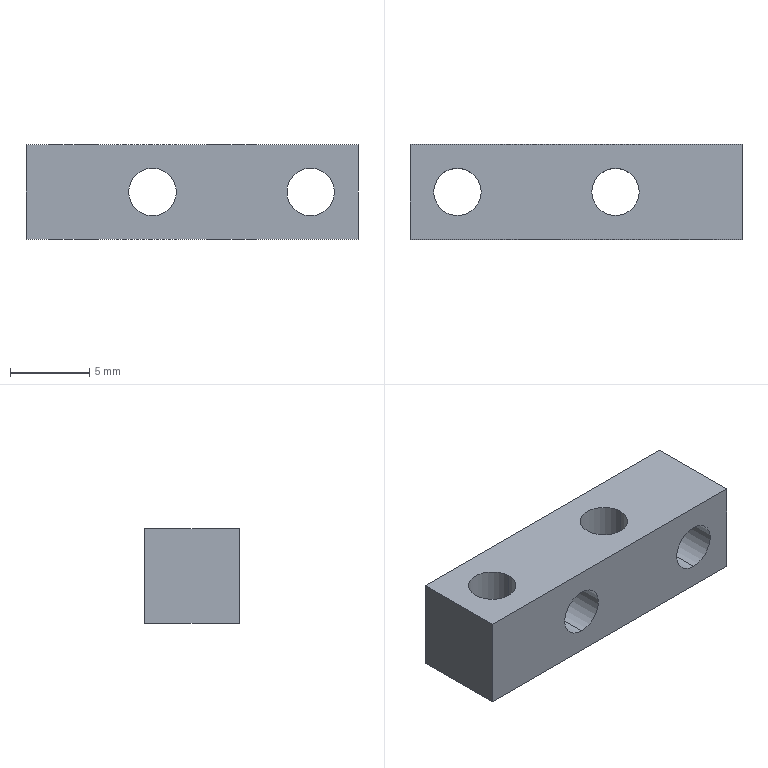Part | SolidWorks | features Extrusion 1, ICE 1 | 1 solid | 14 faces | box 21 x 6 x 6 mm | volume 586.354 mm3 | cylinder 8 | plane 6 | commonest cylinder face diameters 3 x8
STEP:
#1=CARTESIAN_POINT('',(8.,0.,1.5));
#2=VERTEX_POINT('',#1);
#3=CARTESIAN_POINT('',(8.,0.,4.5));
#4=VERTEX_POINT('',#3);
#5=CARTESIAN_POINT('',(8.,0.,3.));
#6=DIRECTION('',(0.,1.,0.));
#7=DIRECTION('',(0.,0.,1.));
#8=AXIS2_PLACEMENT_3D('',#5,#6,#7);
#9=CIRCLE('',#8,1.5);
#10=EDGE_CURVE('',#2,#4,#9,.T.);
#11=ORIENTED_EDGE('',*,*,#10,.F.);
#12=CARTESIAN_POINT('',(8.,6.,1.5));
#13=VERTEX_POINT('',#12);
#14=CARTESIAN_POINT('',(8.,0.,1.5));
#15=DIRECTION('',(0.,1.,0.));
#16=VECTOR('',#15,1000.);
#17=LINE('',#14,#16);
#18=EDGE_CURVE('',#2,#13,#17,.T.);
#19=ORIENTED_EDGE('',*,*,#18,.T.);
#20=CARTESIAN_POINT('',(8.,6.,4.5));
#21=VERTEX_POINT('',#20);
#22=CARTESIAN_POINT('',(8.,6.,3.));
#23=DIRECTION('',(0.,-1.,0.));
#24=DIRECTION('',(0.,0.,-1.));
#25=AXIS2_PLACEMENT_3D('',#22,#23,#24);
#26=CIRCLE('',#25,1.5);
#27=EDGE_CURVE('',#21,#13,#26,.T.);
#28=ORIENTED_EDGE('',*,*,#27,.F.);
#29=CARTESIAN_POINT('',(8.,0.,4.5));
#30=DIRECTION('',(0.,1.,0.));
#31=VECTOR('',#30,1000.);
#32=LINE('',#29,#31);
#33=EDGE_CURVE('',#4,#21,#32,.T.);
#34=ORIENTED_EDGE('',*,*,#33,.F.);
#35=EDGE_LOOP('',(#11,#19,#28,#34));
#36=FACE_OUTER_BOUND('',#35,.T.);
#37=CARTESIAN_POINT('',(8.,0.,3.));
#38=DIRECTION('',(0.,1.,0.));
#39=DIRECTION('',(0.,0.,1.));
#40=AXIS2_PLACEMENT_3D('',#37,#38,#39);
#41=CYLINDRICAL_SURFACE('',#40,1.5);
#42=ADVANCED_FACE('',(#36),#41,.F.);
#43=CARTESIAN_POINT('',(18.,0.,1.5));
#44=VERTEX_POINT('',#43);
#45=CARTESIAN_POINT('',(18.,0.,4.5));
#46=VERTEX_POINT('',#45);
#47=CARTESIAN_POINT('',(18.,0.,3.));
#48=DIRECTION('',(0.,1.,0.));
#49=DIRECTION('',(0.,0.,1.));
#50=AXIS2_PLACEMENT_3D('',#47,#48,#49);
#51=CIRCLE('',#50,1.5);
#52=EDGE_CURVE('',#44,#46,#51,.T.);
#53=ORIENTED_EDGE('',*,*,#52,.F.);
#54=CARTESIAN_POINT('',(18.,6.,1.5));
#55=VERTEX_POINT('',#54);
#56=CARTESIAN_POINT('',(18.,0.,1.5));
#57=DIRECTION('',(0.,1.,0.));
#58=VECTOR('',#57,1000.);
#59=LINE('',#56,#58);
#60=EDGE_CURVE('',#44,#55,#59,.T.);
#61=ORIENTED_EDGE('',*,*,#60,.T.);
#62=CARTESIAN_POINT('',(18.,6.,4.5));
#63=VERTEX_POINT('',#62);
#64=CARTESIAN_POINT('',(18.,6.,3.));
#65=DIRECTION('',(0.,-1.,0.));
#66=DIRECTION('',(0.,0.,-1.));
#67=AXIS2_PLACEMENT_3D('',#64,#65,#66);
#68=CIRCLE('',#67,1.5);
#69=EDGE_CURVE('',#63,#55,#68,.T.);
#70=ORIENTED_EDGE('',*,*,#69,.F.);
#71=CARTESIAN_POINT('',(18.,0.,4.5));
#72=DIRECTION('',(0.,1.,0.));
#73=VECTOR('',#72,1000.);
#74=LINE('',#71,#73);
#75=EDGE_CURVE('',#46,#63,#74,.T.);
#76=ORIENTED_EDGE('',*,*,#75,.F.);
#77=EDGE_LOOP('',(#53,#61,#70,#76));
#78=FACE_OUTER_BOUND('',#77,.T.);
#79=CARTESIAN_POINT('',(18.,0.,3.));
#80=DIRECTION('',(0.,1.,0.));
#81=DIRECTION('',(0.,0.,1.));
#82=AXIS2_PLACEMENT_3D('',#79,#80,#81);
#83=CYLINDRICAL_SURFACE('',#82,1.5);
#84=ADVANCED_FACE('',(#78),#83,.F.);
#85=CARTESIAN_POINT('',(11.5,3.,6.));
#86=VERTEX_POINT('',#85);
#87=CARTESIAN_POINT('',(14.5,3.,6.));
#88=VERTEX_POINT('',#87);
#89=CARTESIAN_POINT('',(13.,3.,6.));
#90=DIRECTION('',(0.,0.,1.));
#91=DIRECTION('',(1.,0.,0.));
#92=AXIS2_PLACEMENT_3D('',#89,#90,#91);
#93=CIRCLE('',#92,1.5);
#94=EDGE_CURVE('',#86,#88,#93,.T.);
#95=ORIENTED_EDGE('',*,*,#94,.T.);
#96=CARTESIAN_POINT('',(14.5,3.,0.));
#97=VERTEX_POINT('',#96);
#98=CARTESIAN_POINT('',(14.5,3.,6.));
#99=DIRECTION('',(0.,0.,-1.));
#100=VECTOR('',#99,1000.);
#101=LINE('',#98,#100);
#102=EDGE_CURVE('',#88,#97,#101,.T.);
#103=ORIENTED_EDGE('',*,*,#102,.T.);
#104=CARTESIAN_POINT('',(11.5,3.,0.));
#105=VERTEX_POINT('',#104);
#106=CARTESIAN_POINT('',(13.,3.,0.));
#107=DIRECTION('',(0.,0.,1.));
#108=DIRECTION('',(1.,0.,0.));
#109=AXIS2_PLACEMENT_3D('',#106,#107,#108);
#110=CIRCLE('',#109,1.5);
#111=EDGE_CURVE('',#105,#97,#110,.T.);
#112=ORIENTED_EDGE('',*,*,#111,.F.);
#113=CARTESIAN_POINT('',(11.5,3.,6.));
#114=DIRECTION('',(0.,0.,-1.));
#115=VECTOR('',#114,1000.);
#116=LINE('',#113,#115);
#117=EDGE_CURVE('',#86,#105,#116,.T.);
#118=ORIENTED_EDGE('',*,*,#117,.F.);
#119=EDGE_LOOP('',(#95,#103,#112,#118));
#120=FACE_OUTER_BOUND('',#119,.T.);
#121=CARTESIAN_POINT('',(13.,3.,6.));
#122=DIRECTION('',(0.,0.,-1.));
#123=DIRECTION('',(-1.,0.,0.));
#124=AXIS2_PLACEMENT_3D('',#121,#122,#123);
#125=CYLINDRICAL_SURFACE('',#124,1.5);
#126=ADVANCED_FACE('',(#120),#125,.F.);
#127=CARTESIAN_POINT('',(1.5,3.,6.));
#128=VERTEX_POINT('',#127);
#129=CARTESIAN_POINT('',(4.5,3.,6.));
#130=VERTEX_POINT('',#129);
#131=CARTESIAN_POINT('',(3.,3.,6.));
#132=DIRECTION('',(0.,0.,1.));
#133=DIRECTION('',(1.,0.,0.));
#134=AXIS2_PLACEMENT_3D('',#131,#132,#133);
#135=CIRCLE('',#134,1.5);
#136=EDGE_CURVE('',#128,#130,#135,.T.);
#137=ORIENTED_EDGE('',*,*,#136,.T.);
#138=CARTESIAN_POINT('',(4.5,3.,0.));
#139=VERTEX_POINT('',#138);
#140=CARTESIAN_POINT('',(4.5,3.,6.));
#141=DIRECTION('',(0.,0.,-1.));
#142=VECTOR('',#141,1000.);
#143=LINE('',#140,#142);
#144=EDGE_CURVE('',#130,#139,#143,.T.);
#145=ORIENTED_EDGE('',*,*,#144,.T.);
#146=CARTESIAN_POINT('',(1.5,3.,0.));
#147=VERTEX_POINT('',#146);
#148=CARTESIAN_POINT('',(3.,3.,0.));
#149=DIRECTION('',(0.,0.,1.));
#150=DIRECTION('',(1.,0.,0.));
#151=AXIS2_PLACEMENT_3D('',#148,#149,#150);
#152=CIRCLE('',#151,1.5);
#153=EDGE_CURVE('',#147,#139,#152,.T.);
#154=ORIENTED_EDGE('',*,*,#153,.F.);
#155=CARTESIAN_POINT('',(1.5,3.,6.));
#156=DIRECTION('',(0.,0.,-1.));
#157=VECTOR('',#156,1000.);
#158=LINE('',#155,#157);
#159=EDGE_CURVE('',#128,#147,#158,.T.);
#160=ORIENTED_EDGE('',*,*,#159,.F.);
#161=EDGE_LOOP('',(#137,#145,#154,#160));
#162=FACE_OUTER_BOUND('',#161,.T.);
#163=CARTESIAN_POINT('',(3.,3.,6.));
#164=DIRECTION('',(0.,0.,-1.));
#165=DIRECTION('',(-1.,0.,0.));
#166=AXIS2_PLACEMENT_3D('',#163,#164,#165);
#167=CYLINDRICAL_SURFACE('',#166,1.5);
#168=ADVANCED_FACE('',(#162),#167,.F.);
#169=CARTESIAN_POINT('',(0.,6.,6.));
#170=VERTEX_POINT('',#169);
#171=CARTESIAN_POINT('',(0.,0.,6.));
#172=VERTEX_POINT('',#171);
#173=CARTESIAN_POINT('',(0.,0.,6.));
#174=DIRECTION('',(0.,-1.,0.));
#175=VECTOR('',#174,1000.);
#176=LINE('',#173,#175);
#177=EDGE_CURVE('',#170,#172,#176,.T.);
#178=ORIENTED_EDGE('',*,*,#177,.T.);
#179=CARTESIAN_POINT('',(21.,0.,6.));
#180=VERTEX_POINT('',#179);
#181=CARTESIAN_POINT('',(0.,0.,6.));
#182=DIRECTION('',(1.,0.,0.));
#183=VECTOR('',#182,1000.);
#184=LINE('',#181,#183);
#185=EDGE_CURVE('',#172,#180,#184,.T.);
#186=ORIENTED_EDGE('',*,*,#185,.T.);
#187=CARTESIAN_POINT('',(21.,6.,6.));
#188=VERTEX_POINT('',#187);
#189=CARTESIAN_POINT('',(21.,0.,6.));
#190=DIRECTION('',(0.,1.,0.));
#191=VECTOR('',#190,1000.);
#192=LINE('',#189,#191);
#193=EDGE_CURVE('',#180,#188,#192,.T.);
#194=ORIENTED_EDGE('',*,*,#193,.T.);
#195=CARTESIAN_POINT('',(0.,6.,6.));
#196=DIRECTION('',(-1.,0.,0.));
#197=VECTOR('',#196,1000.);
#198=LINE('',#195,#197);
#199=EDGE_CURVE('',#188,#170,#198,.T.);
#200=ORIENTED_EDGE('',*,*,#199,.T.);
#201=EDGE_LOOP('',(#178,#186,#194,#200));
#202=FACE_OUTER_BOUND('',#201,.T.);
#203=ORIENTED_EDGE('',*,*,#136,.F.);
#204=CARTESIAN_POINT('',(3.,3.,6.));
#205=DIRECTION('',(0.,0.,1.));
#206=DIRECTION('',(1.,0.,0.));
#207=AXIS2_PLACEMENT_3D('',#204,#205,#206);
#208=CIRCLE('',#207,1.5);
#209=EDGE_CURVE('',#130,#128,#208,.T.);
#210=ORIENTED_EDGE('',*,*,#209,.F.);
#211=EDGE_LOOP('',(#203,#210));
#212=FACE_BOUND('',#211,.T.);
#213=ORIENTED_EDGE('',*,*,#94,.F.);
#214=CARTESIAN_POINT('',(13.,3.,6.));
#215=DIRECTION('',(0.,0.,1.));
#216=DIRECTION('',(1.,0.,0.));
#217=AXIS2_PLACEMENT_3D('',#214,#215,#216);
#218=CIRCLE('',#217,1.5);
#219=EDGE_CURVE('',#88,#86,#218,.T.);
#220=ORIENTED_EDGE('',*,*,#219,.F.);
#221=EDGE_LOOP('',(#213,#220));
#222=FACE_BOUND('',#221,.T.);
#223=CARTESIAN_POINT('',(0.,0.,6.));
#224=DIRECTION('',(0.,0.,-1.));
#225=DIRECTION('',(-1.,0.,0.));
#226=AXIS2_PLACEMENT_3D('',#223,#224,#225);
#227=PLANE('',#226);
#228=ADVANCED_FACE('',(#202,#212,#222),#227,.F.);
#229=ORIENTED_EDGE('',*,*,#153,.T.);
#230=CARTESIAN_POINT('',(3.,3.,0.));
#231=DIRECTION('',(0.,0.,1.));
#232=DIRECTION('',(1.,0.,0.));
#233=AXIS2_PLACEMENT_3D('',#230,#231,#232);
#234=CIRCLE('',#233,1.5);
#235=EDGE_CURVE('',#139,#147,#234,.T.);
#236=ORIENTED_EDGE('',*,*,#235,.T.);
#237=EDGE_LOOP('',(#229,#236));
#238=FACE_BOUND('',#237,.T.);
#239=CARTESIAN_POINT('',(0.,6.,0.));
#240=VERTEX_POINT('',#239);
#241=CARTESIAN_POINT('',(0.,0.,0.));
#242=VERTEX_POINT('',#241);
#243=CARTESIAN_POINT('',(0.,0.,0.));
#244=DIRECTION('',(0.,-1.,0.));
#245=VECTOR('',#244,1000.);
#246=LINE('',#243,#245);
#247=EDGE_CURVE('',#240,#242,#246,.T.);
#248=ORIENTED_EDGE('',*,*,#247,.F.);
#249=CARTESIAN_POINT('',(21.,6.,0.));
#250=VERTEX_POINT('',#249);
#251=CARTESIAN_POINT('',(0.,6.,0.));
#252=DIRECTION('',(-1.,0.,0.));
#253=VECTOR('',#252,1000.);
#254=LINE('',#251,#253);
#255=EDGE_CURVE('',#250,#240,#254,.T.);
#256=ORIENTED_EDGE('',*,*,#255,.F.);
#257=CARTESIAN_POINT('',(21.,0.,0.));
#258=VERTEX_POINT('',#257);
#259=CARTESIAN_POINT('',(21.,0.,0.));
#260=DIRECTION('',(0.,1.,0.));
#261=VECTOR('',#260,1000.);
#262=LINE('',#259,#261);
#263=EDGE_CURVE('',#258,#250,#262,.T.);
#264=ORIENTED_EDGE('',*,*,#263,.F.);
#265=CARTESIAN_POINT('',(0.,0.,0.));
#266=DIRECTION('',(1.,0.,0.));
#267=VECTOR('',#266,1000.);
#268=LINE('',#265,#267);
#269=EDGE_CURVE('',#242,#258,#268,.T.);
#270=ORIENTED_EDGE('',*,*,#269,.F.);
#271=EDGE_LOOP('',(#248,#256,#264,#270));
#272=FACE_OUTER_BOUND('',#271,.T.);
#273=ORIENTED_EDGE('',*,*,#111,.T.);
#274=CARTESIAN_POINT('',(13.,3.,0.));
#275=DIRECTION('',(0.,0.,1.));
#276=DIRECTION('',(1.,0.,0.));
#277=AXIS2_PLACEMENT_3D('',#274,#275,#276);
#278=CIRCLE('',#277,1.5);
#279=EDGE_CURVE('',#97,#105,#278,.T.);
#280=ORIENTED_EDGE('',*,*,#279,.T.);
#281=EDGE_LOOP('',(#273,#280));
#282=FACE_BOUND('',#281,.T.);
#283=CARTESIAN_POINT('',(0.,0.,0.));
#284=DIRECTION('',(0.,0.,-1.));
#285=DIRECTION('',(-1.,0.,0.));
#286=AXIS2_PLACEMENT_3D('',#283,#284,#285);
#287=PLANE('',#286);
#288=ADVANCED_FACE('',(#238,#272,#282),#287,.T.);
#289=ORIENTED_EDGE('',*,*,#247,.T.);
#290=CARTESIAN_POINT('',(0.,0.,6.));
#291=DIRECTION('',(0.,0.,-1.));
#292=VECTOR('',#291,1000.);
#293=LINE('',#290,#292);
#294=EDGE_CURVE('',#172,#242,#293,.T.);
#295=ORIENTED_EDGE('',*,*,#294,.F.);
#296=ORIENTED_EDGE('',*,*,#177,.F.);
#297=CARTESIAN_POINT('',(0.,6.,6.));
#298=DIRECTION('',(0.,0.,-1.));
#299=VECTOR('',#298,1000.);
#300=LINE('',#297,#299);
#301=EDGE_CURVE('',#170,#240,#300,.T.);
#302=ORIENTED_EDGE('',*,*,#301,.T.);
#303=EDGE_LOOP('',(#289,#295,#296,#302));
#304=FACE_OUTER_BOUND('',#303,.T.);
#305=CARTESIAN_POINT('',(0.,0.,6.));
#306=DIRECTION('',(1.,0.,0.));
#307=DIRECTION('',(0.,0.,-1.));
#308=AXIS2_PLACEMENT_3D('',#305,#306,#307);
#309=PLANE('',#308);
#310=ADVANCED_FACE('',(#304),#309,.F.);
#311=CARTESIAN_POINT('',(8.,0.,3.));
#312=DIRECTION('',(0.,1.,0.));
#313=DIRECTION('',(0.,0.,1.));
#314=AXIS2_PLACEMENT_3D('',#311,#312,#313);
#315=CIRCLE('',#314,1.5);
#316=EDGE_CURVE('',#4,#2,#315,.T.);
#317=ORIENTED_EDGE('',*,*,#316,.T.);
#318=ORIENTED_EDGE('',*,*,#10,.T.);
#319=EDGE_LOOP('',(#317,#318));
#320=FACE_BOUND('',#319,.T.);
#321=CARTESIAN_POINT('',(18.,0.,3.));
#322=DIRECTION('',(0.,1.,0.));
#323=DIRECTION('',(0.,0.,1.));
#324=AXIS2_PLACEMENT_3D('',#321,#322,#323);
#325=CIRCLE('',#324,1.5);
#326=EDGE_CURVE('',#46,#44,#325,.T.);
#327=ORIENTED_EDGE('',*,*,#326,.T.);
#328=ORIENTED_EDGE('',*,*,#52,.T.);
#329=EDGE_LOOP('',(#327,#328));
#330=FACE_BOUND('',#329,.T.);
#331=ORIENTED_EDGE('',*,*,#269,.T.);
#332=CARTESIAN_POINT('',(21.,0.,6.));
#333=DIRECTION('',(0.,0.,-1.));
#334=VECTOR('',#333,1000.);
#335=LINE('',#332,#334);
#336=EDGE_CURVE('',#180,#258,#335,.T.);
#337=ORIENTED_EDGE('',*,*,#336,.F.);
#338=ORIENTED_EDGE('',*,*,#185,.F.);
#339=ORIENTED_EDGE('',*,*,#294,.T.);
#340=EDGE_LOOP('',(#331,#337,#338,#339));
#341=FACE_OUTER_BOUND('',#340,.T.);
#342=CARTESIAN_POINT('',(0.,0.,6.));
#343=DIRECTION('',(0.,1.,0.));
#344=DIRECTION('',(0.,0.,1.));
#345=AXIS2_PLACEMENT_3D('',#342,#343,#344);
#346=PLANE('',#345);
#347=ADVANCED_FACE('',(#320,#330,#341),#346,.F.);
#348=ORIENTED_EDGE('',*,*,#263,.T.);
#349=CARTESIAN_POINT('',(21.,6.,6.));
#350=DIRECTION('',(0.,0.,-1.));
#351=VECTOR('',#350,1000.);
#352=LINE('',#349,#351);
#353=EDGE_CURVE('',#188,#250,#352,.T.);
#354=ORIENTED_EDGE('',*,*,#353,.F.);
#355=ORIENTED_EDGE('',*,*,#193,.F.);
#356=ORIENTED_EDGE('',*,*,#336,.T.);
#357=EDGE_LOOP('',(#348,#354,#355,#356));
#358=FACE_OUTER_BOUND('',#357,.T.);
#359=CARTESIAN_POINT('',(21.,0.,6.));
#360=DIRECTION('',(-1.,0.,0.));
#361=DIRECTION('',(0.,0.,1.));
#362=AXIS2_PLACEMENT_3D('',#359,#360,#361);
#363=PLANE('',#362);
#364=ADVANCED_FACE('',(#358),#363,.F.);
#365=ORIENTED_EDGE('',*,*,#27,.T.);
#366=CARTESIAN_POINT('',(8.,6.,3.));
#367=DIRECTION('',(0.,-1.,0.));
#368=DIRECTION('',(0.,0.,-1.));
#369=AXIS2_PLACEMENT_3D('',#366,#367,#368);
#370=CIRCLE('',#369,1.5);
#371=EDGE_CURVE('',#13,#21,#370,.T.);
#372=ORIENTED_EDGE('',*,*,#371,.T.);
#373=EDGE_LOOP('',(#365,#372));
#374=FACE_BOUND('',#373,.T.);
#375=ORIENTED_EDGE('',*,*,#69,.T.);
#376=CARTESIAN_POINT('',(18.,6.,3.));
#377=DIRECTION('',(0.,-1.,0.));
#378=DIRECTION('',(0.,0.,-1.));
#379=AXIS2_PLACEMENT_3D('',#376,#377,#378);
#380=CIRCLE('',#379,1.5);
#381=EDGE_CURVE('',#55,#63,#380,.T.);
#382=ORIENTED_EDGE('',*,*,#381,.T.);
#383=EDGE_LOOP('',(#375,#382));
#384=FACE_BOUND('',#383,.T.);
#385=ORIENTED_EDGE('',*,*,#255,.T.);
#386=ORIENTED_EDGE('',*,*,#301,.F.);
#387=ORIENTED_EDGE('',*,*,#199,.F.);
#388=ORIENTED_EDGE('',*,*,#353,.T.);
#389=EDGE_LOOP('',(#385,#386,#387,#388));
#390=FACE_OUTER_BOUND('',#389,.T.);
#391=CARTESIAN_POINT('',(0.,6.,6.));
#392=DIRECTION('',(0.,-1.,0.));
#393=DIRECTION('',(0.,0.,-1.));
#394=AXIS2_PLACEMENT_3D('',#391,#392,#393);
#395=PLANE('',#394);
#396=ADVANCED_FACE('',(#374,#384,#390),#395,.F.);
#397=ORIENTED_EDGE('',*,*,#144,.F.);
#398=ORIENTED_EDGE('',*,*,#209,.T.);
#399=ORIENTED_EDGE('',*,*,#159,.T.);
#400=ORIENTED_EDGE('',*,*,#235,.F.);
#401=EDGE_LOOP('',(#397,#398,#399,#400));
#402=FACE_OUTER_BOUND('',#401,.T.);
#403=CARTESIAN_POINT('',(3.,3.,6.));
#404=DIRECTION('',(0.,0.,-1.));
#405=DIRECTION('',(-1.,0.,0.));
#406=AXIS2_PLACEMENT_3D('',#403,#404,#405);
#407=CYLINDRICAL_SURFACE('',#406,1.5);
#408=ADVANCED_FACE('',(#402),#407,.F.);
#409=ORIENTED_EDGE('',*,*,#102,.F.);
#410=ORIENTED_EDGE('',*,*,#219,.T.);
#411=ORIENTED_EDGE('',*,*,#117,.T.);
#412=ORIENTED_EDGE('',*,*,#279,.F.);
#413=EDGE_LOOP('',(#409,#410,#411,#412));
#414=FACE_OUTER_BOUND('',#413,.T.);
#415=CARTESIAN_POINT('',(13.,3.,6.));
#416=DIRECTION('',(0.,0.,-1.));
#417=DIRECTION('',(-1.,0.,0.));
#418=AXIS2_PLACEMENT_3D('',#415,#416,#417);
#419=CYLINDRICAL_SURFACE('',#418,1.5);
#420=ADVANCED_FACE('',(#414),#419,.F.);
#421=ORIENTED_EDGE('',*,*,#60,.F.);
#422=ORIENTED_EDGE('',*,*,#326,.F.);
#423=ORIENTED_EDGE('',*,*,#75,.T.);
#424=ORIENTED_EDGE('',*,*,#381,.F.);
#425=EDGE_LOOP('',(#421,#422,#423,#424));
#426=FACE_OUTER_BOUND('',#425,.T.);
#427=CARTESIAN_POINT('',(18.,0.,3.));
#428=DIRECTION('',(0.,1.,0.));
#429=DIRECTION('',(0.,0.,1.));
#430=AXIS2_PLACEMENT_3D('',#427,#428,#429);
#431=CYLINDRICAL_SURFACE('',#430,1.5);
#432=ADVANCED_FACE('',(#426),#431,.F.);
#433=ORIENTED_EDGE('',*,*,#18,.F.);
#434=ORIENTED_EDGE('',*,*,#316,.F.);
#435=ORIENTED_EDGE('',*,*,#33,.T.);
#436=ORIENTED_EDGE('',*,*,#371,.F.);
#437=EDGE_LOOP('',(#433,#434,#435,#436));
#438=FACE_OUTER_BOUND('',#437,.T.);
#439=CARTESIAN_POINT('',(8.,0.,3.));
#440=DIRECTION('',(0.,1.,0.));
#441=DIRECTION('',(0.,0.,1.));
#442=AXIS2_PLACEMENT_3D('',#439,#440,#441);
#443=CYLINDRICAL_SURFACE('',#442,1.5);
#444=ADVANCED_FACE('',(#438),#443,.F.);
#445=CLOSED_SHELL('',(#42,#84,#126,#168,#228,#288,#310,#347,#364,#396,#408,#420,#432,#444));
#446=MANIFOLD_SOLID_BREP('',#445);
#447=CARTESIAN_POINT('',(0.,0.,0.));
#448=DIRECTION('',(0.,0.,1.));
#449=DIRECTION('',(1.,0.,0.));
#450=AXIS2_PLACEMENT_3D('',#447,#448,#449);
#451=(LENGTH_UNIT()NAMED_UNIT(*)SI_UNIT(.MILLI.,.METRE.));
#452=UNCERTAINTY_MEASURE_WITH_UNIT(LENGTH_MEASURE(0.00001),#451,'','');
#453=(NAMED_UNIT(*)PLANE_ANGLE_UNIT()SI_UNIT($,.RADIAN.));
#454=(NAMED_UNIT(*)SI_UNIT($,.STERADIAN.)SOLID_ANGLE_UNIT());
#455=(GEOMETRIC_REPRESENTATION_CONTEXT(3)GLOBAL_UNCERTAINTY_ASSIGNED_CONTEXT((#452))GLOBAL_UNIT_ASSIGNED_CONTEXT((#451,#453,#454))REPRESENTATION_CONTEXT('',''));
#456=ADVANCED_BREP_SHAPE_REPRESENTATION('',(#446,#450),#455);